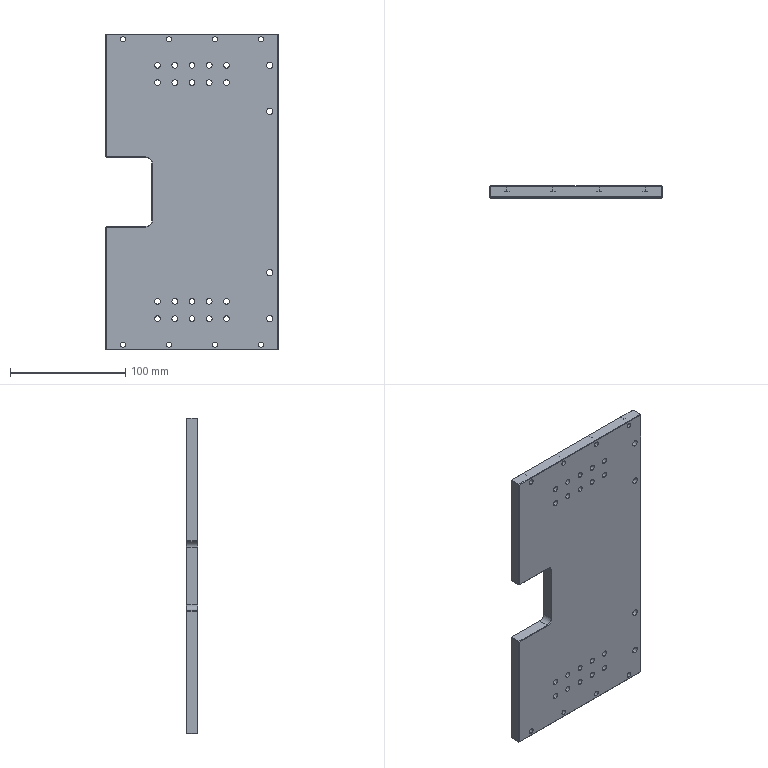Part | STEP file | BPSP-11-004Unloading Support Plate3_Default | 1 solid | 150 faces | box 150 x 10 x 274 mm | volume 378327 mm3 | cylinder 90 | plane 56 | cone 4 | commonest cylinder face diameters 5 x40 4.5 x16 8 x16 10 x10 5.5 x8